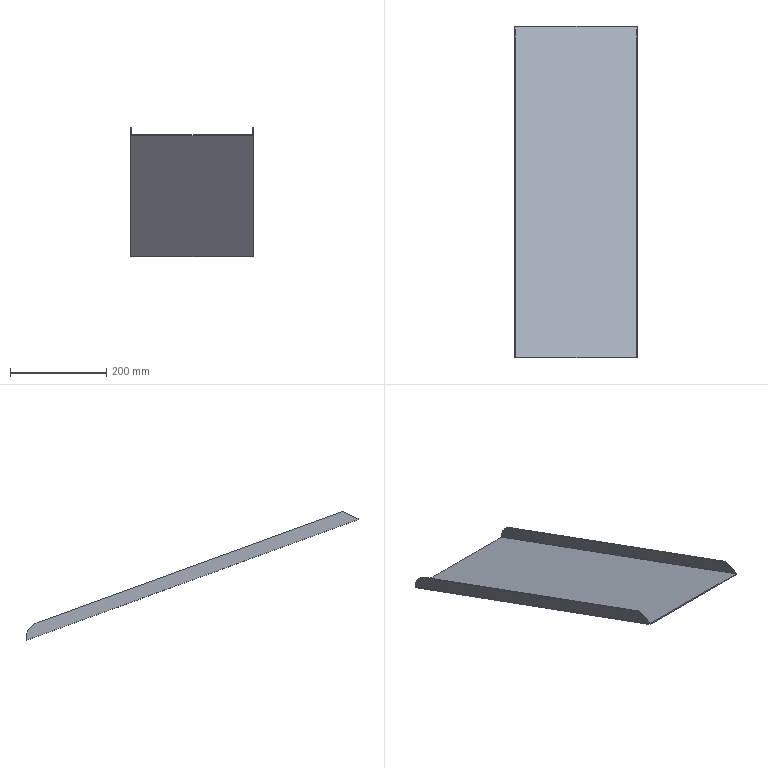Part | NX | features solid 2 | 1 solid | 14 faces | box 255 x 690 x 268.21 mm | volume 445770 mm3 | plane 12 | cylinder 2 | commonest cylinder face diameters 70 x2
STEP:
#1=CARTESIAN_POINT('',(-857.,620.,-449.011));
#2=VERTEX_POINT('',#1);
#3=CARTESIAN_POINT('',(-1108.,620.,-449.011));
#4=VERTEX_POINT('',#3);
#5=CARTESIAN_POINT('',(-855.,620.,-449.011));
#6=DIRECTION('',(-1.,0.,0.));
#7=VECTOR('',#6,1000.);
#8=LINE('',#5,#7);
#9=EDGE_CURVE('',#2,#4,#8,.T.);
#10=ORIENTED_EDGE('',*,*,#9,.T.);
#11=CARTESIAN_POINT('',(-1108.,-70.,-197.872));
#12=VERTEX_POINT('',#11);
#13=CARTESIAN_POINT('',(-1108.,-70.,-197.872));
#14=DIRECTION('',(0.,0.9397,-0.342));
#15=VECTOR('',#14,1000.);
#16=LINE('',#13,#15);
#17=EDGE_CURVE('',#12,#4,#16,.T.);
#18=ORIENTED_EDGE('',*,*,#17,.F.);
#19=CARTESIAN_POINT('',(-857.,-70.,-197.872));
#20=VERTEX_POINT('',#19);
#21=CARTESIAN_POINT('',(-855.,-70.,-197.872));
#22=DIRECTION('',(1.,0.,0.));
#23=VECTOR('',#22,1000.);
#24=LINE('',#21,#23);
#25=EDGE_CURVE('',#20,#12,#24,.F.);
#26=ORIENTED_EDGE('',*,*,#25,.F.);
#27=CARTESIAN_POINT('',(-857.,-70.,-197.872));
#28=DIRECTION('',(0.,0.9397,-0.342));
#29=VECTOR('',#28,1000.);
#30=LINE('',#27,#29);
#31=EDGE_CURVE('',#20,#2,#30,.T.);
#32=ORIENTED_EDGE('',*,*,#31,.T.);
#33=EDGE_LOOP('',(#10,#18,#26,#32));
#34=FACE_BOUND('',#33,.T.);
#35=CARTESIAN_POINT('',(-855.,-69.316,-198.121));
#36=DIRECTION('',(0.,-0.342,-0.9397));
#37=DIRECTION('',(-1.,0.,0.));
#38=AXIS2_PLACEMENT_3D('',#35,#36,#37);
#39=PLANE('',#38);
#40=ADVANCED_FACE('',(#34),#39,.F.);
#41=CARTESIAN_POINT('',(-857.,620.,-446.914));
#42=VERTEX_POINT('',#41);
#43=CARTESIAN_POINT('',(-857.,620.,-570.));
#44=DIRECTION('',(0.,0.,1.));
#45=VECTOR('',#44,1000.);
#46=LINE('',#43,#45);
#47=EDGE_CURVE('',#2,#42,#46,.T.);
#48=ORIENTED_EDGE('',*,*,#47,.T.);
#49=CARTESIAN_POINT('',(-855.,620.,-446.914));
#50=VERTEX_POINT('',#49);
#51=CARTESIAN_POINT('',(50.,620.,-446.914));
#52=DIRECTION('',(-1.,0.,0.));
#53=VECTOR('',#52,1000.);
#54=LINE('',#51,#53);
#55=EDGE_CURVE('',#42,#50,#54,.F.);
#56=ORIENTED_EDGE('',*,*,#55,.T.);
#57=CARTESIAN_POINT('',(-855.,620.,-451.139));
#58=VERTEX_POINT('',#57);
#59=CARTESIAN_POINT('',(-855.,620.,-570.));
#60=DIRECTION('',(0.,0.,-1.));
#61=VECTOR('',#60,1000.);
#62=LINE('',#59,#61);
#63=EDGE_CURVE('',#50,#58,#62,.T.);
#64=ORIENTED_EDGE('',*,*,#63,.T.);
#65=CARTESIAN_POINT('',(-1110.,620.,-451.139));
#66=VERTEX_POINT('',#65);
#67=CARTESIAN_POINT('',(-855.,620.,-451.139));
#68=DIRECTION('',(-1.,0.,0.));
#69=VECTOR('',#68,1000.);
#70=LINE('',#67,#69);
#71=EDGE_CURVE('',#58,#66,#70,.T.);
#72=ORIENTED_EDGE('',*,*,#71,.T.);
#73=CARTESIAN_POINT('',(-1110.,620.,-446.914));
#74=VERTEX_POINT('',#73);
#75=CARTESIAN_POINT('',(-1110.,620.,-570.));
#76=DIRECTION('',(0.,0.,-1.));
#77=VECTOR('',#76,1000.);
#78=LINE('',#75,#77);
#79=EDGE_CURVE('',#74,#66,#78,.T.);
#80=ORIENTED_EDGE('',*,*,#79,.F.);
#81=CARTESIAN_POINT('',(-1108.,620.,-446.914));
#82=VERTEX_POINT('',#81);
#83=CARTESIAN_POINT('',(50.,620.,-446.914));
#84=DIRECTION('',(-1.,0.,0.));
#85=VECTOR('',#84,1000.);
#86=LINE('',#83,#85);
#87=EDGE_CURVE('',#74,#82,#86,.F.);
#88=ORIENTED_EDGE('',*,*,#87,.T.);
#89=CARTESIAN_POINT('',(-1108.,620.,-570.));
#90=DIRECTION('',(0.,0.,1.));
#91=VECTOR('',#90,1000.);
#92=LINE('',#89,#91);
#93=EDGE_CURVE('',#4,#82,#92,.T.);
#94=ORIENTED_EDGE('',*,*,#93,.F.);
#95=ORIENTED_EDGE('',*,*,#9,.F.);
#96=EDGE_LOOP('',(#48,#56,#64,#72,#80,#88,#94,#95));
#97=FACE_BOUND('',#96,.T.);
#98=CARTESIAN_POINT('',(50.,620.,-570.));
#99=DIRECTION('',(0.,-1.,0.));
#100=DIRECTION('',(-1.,0.,0.));
#101=AXIS2_PLACEMENT_3D('',#98,#99,#100);
#102=PLANE('',#101);
#103=ADVANCED_FACE('',(#97),#102,.F.);
#104=CARTESIAN_POINT('',(-855.,-37.957,-182.93));
#105=VERTEX_POINT('',#104);
#106=CARTESIAN_POINT('',(-855.,596.971,-414.025));
#107=VERTEX_POINT('',#106);
#108=CARTESIAN_POINT('',(-855.,-61.449,-174.379));
#109=DIRECTION('',(0.,0.9397,-0.342));
#110=VECTOR('',#109,1000.);
#111=LINE('',#108,#110);
#112=EDGE_CURVE('',#105,#107,#111,.T.);
#113=ORIENTED_EDGE('',*,*,#112,.F.);
#114=CARTESIAN_POINT('',(-855.,-70.,-197.872));
#115=VERTEX_POINT('',#114);
#116=CARTESIAN_POINT('',(-855.,-70.,-197.872));
#117=DIRECTION('',(0.,0.9063,0.4226));
#118=VECTOR('',#117,1000.);
#119=LINE('',#116,#118);
#120=EDGE_CURVE('',#105,#115,#119,.F.);
#121=ORIENTED_EDGE('',*,*,#120,.T.);
#122=CARTESIAN_POINT('',(-855.,-70.,-200.));
#123=VERTEX_POINT('',#122);
#124=CARTESIAN_POINT('',(-855.,-70.,0.00000074));
#125=DIRECTION('',(0.,0.,1.));
#126=VECTOR('',#125,1000.);
#127=LINE('',#124,#126);
#128=EDGE_CURVE('',#115,#123,#127,.F.);
#129=ORIENTED_EDGE('',*,*,#128,.T.);
#130=CARTESIAN_POINT('',(-855.,-70.,-200.));
#131=DIRECTION('',(0.,0.9397,-0.342));
#132=VECTOR('',#131,1000.);
#133=LINE('',#130,#132);
#134=EDGE_CURVE('',#123,#58,#133,.T.);
#135=ORIENTED_EDGE('',*,*,#134,.T.);
#136=ORIENTED_EDGE('',*,*,#63,.F.);
#137=CARTESIAN_POINT('',(-855.,585.,-446.914));
#138=DIRECTION('',(-1.,0.,0.));
#139=DIRECTION('',(0.,0.,1.));
#140=AXIS2_PLACEMENT_3D('',#137,#138,#139);
#141=CIRCLE('',#140,35.);
#142=EDGE_CURVE('',#50,#107,#141,.F.);
#143=ORIENTED_EDGE('',*,*,#142,.T.);
#144=EDGE_LOOP('',(#113,#121,#129,#135,#136,#143));
#145=FACE_BOUND('',#144,.T.);
#146=CARTESIAN_POINT('',(-855.,-69.316,-198.121));
#147=DIRECTION('',(-1.,0.,0.));
#148=DIRECTION('',(0.,0.,1.));
#149=AXIS2_PLACEMENT_3D('',#146,#147,#148);
#150=PLANE('',#149);
#151=ADVANCED_FACE('',(#145),#150,.F.);
#152=CARTESIAN_POINT('',(-1110.,-70.,-200.));
#153=VERTEX_POINT('',#152);
#154=CARTESIAN_POINT('',(-855.,-70.,-200.));
#155=DIRECTION('',(1.,0.,0.));
#156=VECTOR('',#155,1000.);
#157=LINE('',#154,#156);
#158=EDGE_CURVE('',#123,#153,#157,.F.);
#159=ORIENTED_EDGE('',*,*,#158,.F.);
#160=ORIENTED_EDGE('',*,*,#128,.F.);
#161=CARTESIAN_POINT('',(-855.,-70.,-197.872));
#162=DIRECTION('',(1.,0.,0.));
#163=VECTOR('',#162,1000.);
#164=LINE('',#161,#163);
#165=EDGE_CURVE('',#115,#20,#164,.F.);
#166=ORIENTED_EDGE('',*,*,#165,.T.);
#167=ORIENTED_EDGE('',*,*,#25,.T.);
#168=CARTESIAN_POINT('',(-1110.,-70.,-197.872));
#169=VERTEX_POINT('',#168);
#170=CARTESIAN_POINT('',(-1108.,-70.,-197.872));
#171=DIRECTION('',(1.,0.,0.));
#172=VECTOR('',#171,1000.);
#173=LINE('',#170,#172);
#174=EDGE_CURVE('',#12,#169,#173,.F.);
#175=ORIENTED_EDGE('',*,*,#174,.T.);
#176=CARTESIAN_POINT('',(-1110.,-70.,0.000000796));
#177=DIRECTION('',(0.,0.,1.));
#178=VECTOR('',#177,1000.);
#179=LINE('',#176,#178);
#180=EDGE_CURVE('',#169,#153,#179,.F.);
#181=ORIENTED_EDGE('',*,*,#180,.T.);
#182=EDGE_LOOP('',(#159,#160,#166,#167,#175,#181));
#183=FACE_BOUND('',#182,.T.);
#184=CARTESIAN_POINT('',(2540.,-70.,0.));
#185=DIRECTION('',(0.,1.,0.));
#186=DIRECTION('',(0.,0.,1.));
#187=AXIS2_PLACEMENT_3D('',#184,#185,#186);
#188=PLANE('',#187);
#189=ADVANCED_FACE('',(#183),#188,.F.);
#190=ORIENTED_EDGE('',*,*,#180,.F.);
#191=CARTESIAN_POINT('',(-1110.,-37.957,-182.93));
#192=VERTEX_POINT('',#191);
#193=CARTESIAN_POINT('',(-1110.,-69.533,-197.654));
#194=DIRECTION('',(0.,-0.9063,-0.4226));
#195=VECTOR('',#194,1000.);
#196=LINE('',#193,#195);
#197=EDGE_CURVE('',#169,#192,#196,.F.);
#198=ORIENTED_EDGE('',*,*,#197,.T.);
#199=CARTESIAN_POINT('',(-1110.,596.971,-414.025));
#200=VERTEX_POINT('',#199);
#201=CARTESIAN_POINT('',(-1110.,-61.449,-174.379));
#202=DIRECTION('',(0.,0.9397,-0.342));
#203=VECTOR('',#202,1000.);
#204=LINE('',#201,#203);
#205=EDGE_CURVE('',#192,#200,#204,.T.);
#206=ORIENTED_EDGE('',*,*,#205,.T.);
#207=CARTESIAN_POINT('',(-1110.,585.,-446.914));
#208=DIRECTION('',(-1.,0.,0.));
#209=DIRECTION('',(0.,0.,1.));
#210=AXIS2_PLACEMENT_3D('',#207,#208,#209);
#211=CIRCLE('',#210,35.);
#212=EDGE_CURVE('',#200,#74,#211,.T.);
#213=ORIENTED_EDGE('',*,*,#212,.T.);
#214=ORIENTED_EDGE('',*,*,#79,.T.);
#215=CARTESIAN_POINT('',(-1110.,-70.,-200.));
#216=DIRECTION('',(0.,-0.9397,0.342));
#217=VECTOR('',#216,1000.);
#218=LINE('',#215,#217);
#219=EDGE_CURVE('',#153,#66,#218,.F.);
#220=ORIENTED_EDGE('',*,*,#219,.F.);
#221=EDGE_LOOP('',(#190,#198,#206,#213,#214,#220));
#222=FACE_BOUND('',#221,.T.);
#223=CARTESIAN_POINT('',(-1110.,-69.316,-198.121));
#224=DIRECTION('',(-1.,0.,0.));
#225=DIRECTION('',(0.,0.,1.));
#226=AXIS2_PLACEMENT_3D('',#223,#224,#225);
#227=PLANE('',#226);
#228=ADVANCED_FACE('',(#222),#227,.T.);
#229=ORIENTED_EDGE('',*,*,#71,.F.);
#230=ORIENTED_EDGE('',*,*,#134,.F.);
#231=ORIENTED_EDGE('',*,*,#158,.T.);
#232=ORIENTED_EDGE('',*,*,#219,.T.);
#233=EDGE_LOOP('',(#229,#230,#231,#232));
#234=FACE_BOUND('',#233,.T.);
#235=CARTESIAN_POINT('',(-855.,-70.,-200.));
#236=DIRECTION('',(0.,-0.342,-0.9397));
#237=DIRECTION('',(-1.,0.,0.));
#238=AXIS2_PLACEMENT_3D('',#235,#236,#237);
#239=PLANE('',#238);
#240=ADVANCED_FACE('',(#234),#239,.T.);
#241=CARTESIAN_POINT('',(-857.,-37.957,-182.93));
#242=VERTEX_POINT('',#241);
#243=CARTESIAN_POINT('',(-857.,596.971,-414.025));
#244=VERTEX_POINT('',#243);
#245=CARTESIAN_POINT('',(-857.,-61.449,-174.379));
#246=DIRECTION('',(0.,0.9397,-0.342));
#247=VECTOR('',#246,1000.);
#248=LINE('',#245,#247);
#249=EDGE_CURVE('',#242,#244,#248,.T.);
#250=ORIENTED_EDGE('',*,*,#249,.F.);
#251=CARTESIAN_POINT('',(-855.,-37.957,-182.93));
#252=DIRECTION('',(1.,0.,0.));
#253=VECTOR('',#252,1000.);
#254=LINE('',#251,#253);
#255=EDGE_CURVE('',#242,#105,#254,.T.);
#256=ORIENTED_EDGE('',*,*,#255,.T.);
#257=ORIENTED_EDGE('',*,*,#112,.T.);
#258=CARTESIAN_POINT('',(-855.,596.971,-414.025));
#259=DIRECTION('',(-1.,0.,0.));
#260=VECTOR('',#259,1000.);
#261=LINE('',#258,#260);
#262=EDGE_CURVE('',#107,#244,#261,.T.);
#263=ORIENTED_EDGE('',*,*,#262,.T.);
#264=EDGE_LOOP('',(#250,#256,#257,#263));
#265=FACE_BOUND('',#264,.T.);
#266=CARTESIAN_POINT('',(-855.,-61.449,-174.379));
#267=DIRECTION('',(0.,-0.342,-0.9397));
#268=DIRECTION('',(0.,0.9397,-0.342));
#269=AXIS2_PLACEMENT_3D('',#266,#267,#268);
#270=PLANE('',#269);
#271=ADVANCED_FACE('',(#265),#270,.F.);
#272=ORIENTED_EDGE('',*,*,#31,.F.);
#273=CARTESIAN_POINT('',(-857.,-70.,-197.872));
#274=DIRECTION('',(0.,-0.9063,-0.4226));
#275=VECTOR('',#274,1000.);
#276=LINE('',#273,#275);
#277=EDGE_CURVE('',#20,#242,#276,.F.);
#278=ORIENTED_EDGE('',*,*,#277,.T.);
#279=ORIENTED_EDGE('',*,*,#249,.T.);
#280=CARTESIAN_POINT('',(-857.,585.,-446.914));
#281=DIRECTION('',(1.,0.,0.));
#282=DIRECTION('',(0.,0.,-1.));
#283=AXIS2_PLACEMENT_3D('',#280,#281,#282);
#284=CIRCLE('',#283,35.);
#285=EDGE_CURVE('',#244,#42,#284,.F.);
#286=ORIENTED_EDGE('',*,*,#285,.T.);
#287=ORIENTED_EDGE('',*,*,#47,.F.);
#288=EDGE_LOOP('',(#272,#278,#279,#286,#287));
#289=FACE_BOUND('',#288,.T.);
#290=CARTESIAN_POINT('',(-857.,-70.,-197.872));
#291=DIRECTION('',(1.,0.,0.));
#292=DIRECTION('',(0.,0.,-1.));
#293=AXIS2_PLACEMENT_3D('',#290,#291,#292);
#294=PLANE('',#293);
#295=ADVANCED_FACE('',(#289),#294,.F.);
#296=ORIENTED_EDGE('',*,*,#205,.F.);
#297=CARTESIAN_POINT('',(-1108.,-37.957,-182.93));
#298=VERTEX_POINT('',#297);
#299=CARTESIAN_POINT('',(-1108.,-37.957,-182.93));
#300=DIRECTION('',(1.,0.,0.));
#301=VECTOR('',#300,1000.);
#302=LINE('',#299,#301);
#303=EDGE_CURVE('',#192,#298,#302,.T.);
#304=ORIENTED_EDGE('',*,*,#303,.T.);
#305=CARTESIAN_POINT('',(-1108.,596.971,-414.025));
#306=VERTEX_POINT('',#305);
#307=CARTESIAN_POINT('',(-1108.,-61.449,-174.379));
#308=DIRECTION('',(0.,0.9397,-0.342));
#309=VECTOR('',#308,1000.);
#310=LINE('',#307,#309);
#311=EDGE_CURVE('',#298,#306,#310,.T.);
#312=ORIENTED_EDGE('',*,*,#311,.T.);
#313=CARTESIAN_POINT('',(-1108.,596.971,-414.025));
#314=DIRECTION('',(-1.,0.,0.));
#315=VECTOR('',#314,1000.);
#316=LINE('',#313,#315);
#317=EDGE_CURVE('',#306,#200,#316,.T.);
#318=ORIENTED_EDGE('',*,*,#317,.T.);
#319=EDGE_LOOP('',(#296,#304,#312,#318));
#320=FACE_BOUND('',#319,.T.);
#321=CARTESIAN_POINT('',(-1108.,-61.449,-174.379));
#322=DIRECTION('',(0.,-0.342,-0.9397));
#323=DIRECTION('',(0.,0.9397,-0.342));
#324=AXIS2_PLACEMENT_3D('',#321,#322,#323);
#325=PLANE('',#324);
#326=ADVANCED_FACE('',(#320),#325,.F.);
#327=ORIENTED_EDGE('',*,*,#311,.F.);
#328=CARTESIAN_POINT('',(-1108.,-70.,-197.872));
#329=DIRECTION('',(0.,0.9063,0.4226));
#330=VECTOR('',#329,1000.);
#331=LINE('',#328,#330);
#332=EDGE_CURVE('',#298,#12,#331,.F.);
#333=ORIENTED_EDGE('',*,*,#332,.T.);
#334=ORIENTED_EDGE('',*,*,#17,.T.);
#335=ORIENTED_EDGE('',*,*,#93,.T.);
#336=CARTESIAN_POINT('',(-1108.,585.,-446.914));
#337=DIRECTION('',(1.,0.,0.));
#338=DIRECTION('',(0.,0.,-1.));
#339=AXIS2_PLACEMENT_3D('',#336,#337,#338);
#340=CIRCLE('',#339,35.);
#341=EDGE_CURVE('',#82,#306,#340,.T.);
#342=ORIENTED_EDGE('',*,*,#341,.T.);
#343=EDGE_LOOP('',(#327,#333,#334,#335,#342));
#344=FACE_BOUND('',#343,.T.);
#345=CARTESIAN_POINT('',(-1108.,-70.,-197.872));
#346=DIRECTION('',(1.,0.,0.));
#347=DIRECTION('',(0.,0.,-1.));
#348=AXIS2_PLACEMENT_3D('',#345,#346,#347);
#349=PLANE('',#348);
#350=ADVANCED_FACE('',(#344),#349,.T.);
#351=ORIENTED_EDGE('',*,*,#341,.F.);
#352=ORIENTED_EDGE('',*,*,#87,.F.);
#353=ORIENTED_EDGE('',*,*,#212,.F.);
#354=ORIENTED_EDGE('',*,*,#317,.F.);
#355=EDGE_LOOP('',(#351,#352,#353,#354));
#356=FACE_BOUND('',#355,.T.);
#357=CARTESIAN_POINT('',(-1108.,585.,-446.914));
#358=DIRECTION('',(-1.,0.,0.));
#359=DIRECTION('',(0.,0.,1.));
#360=AXIS2_PLACEMENT_3D('',#357,#358,#359);
#361=CYLINDRICAL_SURFACE('',#360,35.);
#362=ADVANCED_FACE('',(#356),#361,.T.);
#363=ORIENTED_EDGE('',*,*,#142,.F.);
#364=ORIENTED_EDGE('',*,*,#55,.F.);
#365=ORIENTED_EDGE('',*,*,#285,.F.);
#366=ORIENTED_EDGE('',*,*,#262,.F.);
#367=EDGE_LOOP('',(#363,#364,#365,#366));
#368=FACE_BOUND('',#367,.T.);
#369=CARTESIAN_POINT('',(-855.,585.,-446.914));
#370=DIRECTION('',(-1.,0.,0.));
#371=DIRECTION('',(0.,0.,1.));
#372=AXIS2_PLACEMENT_3D('',#369,#370,#371);
#373=CYLINDRICAL_SURFACE('',#372,35.);
#374=ADVANCED_FACE('',(#368),#373,.T.);
#375=ORIENTED_EDGE('',*,*,#332,.F.);
#376=ORIENTED_EDGE('',*,*,#303,.F.);
#377=ORIENTED_EDGE('',*,*,#197,.F.);
#378=ORIENTED_EDGE('',*,*,#174,.F.);
#379=EDGE_LOOP('',(#375,#376,#377,#378));
#380=FACE_BOUND('',#379,.T.);
#381=CARTESIAN_POINT('',(-1108.,-70.,-197.872));
#382=DIRECTION('',(0.,0.4226,-0.9063));
#383=DIRECTION('',(0.,0.9063,0.4226));
#384=AXIS2_PLACEMENT_3D('',#381,#382,#383);
#385=PLANE('',#384);
#386=ADVANCED_FACE('',(#380),#385,.F.);
#387=ORIENTED_EDGE('',*,*,#120,.F.);
#388=ORIENTED_EDGE('',*,*,#255,.F.);
#389=ORIENTED_EDGE('',*,*,#277,.F.);
#390=ORIENTED_EDGE('',*,*,#165,.F.);
#391=EDGE_LOOP('',(#387,#388,#389,#390));
#392=FACE_BOUND('',#391,.T.);
#393=CARTESIAN_POINT('',(-855.,-70.,-197.872));
#394=DIRECTION('',(0.,0.4226,-0.9063));
#395=DIRECTION('',(0.,0.9063,0.4226));
#396=AXIS2_PLACEMENT_3D('',#393,#394,#395);
#397=PLANE('',#396);
#398=ADVANCED_FACE('',(#392),#397,.F.);
#399=CLOSED_SHELL('',(#40,#103,#151,#189,#228,#240,#271,#295,#326,#350,#362,#374,#386,#398));
#400=MANIFOLD_SOLID_BREP('',#399);
#401=(LENGTH_UNIT()NAMED_UNIT(*)SI_UNIT(.MILLI.,.METRE.));
#402=UNCERTAINTY_MEASURE_WITH_UNIT(LENGTH_MEASURE(0.00001),#401,'','');
#403=(NAMED_UNIT(*)PLANE_ANGLE_UNIT()SI_UNIT($,.RADIAN.));
#404=(NAMED_UNIT(*)SI_UNIT($,.STERADIAN.)SOLID_ANGLE_UNIT());
#405=(GEOMETRIC_REPRESENTATION_CONTEXT(3)GLOBAL_UNCERTAINTY_ASSIGNED_CONTEXT((#402))GLOBAL_UNIT_ASSIGNED_CONTEXT((#401,#403,#404))REPRESENTATION_CONTEXT('',''));
#406=ADVANCED_BREP_SHAPE_REPRESENTATION('',(#400),#405);